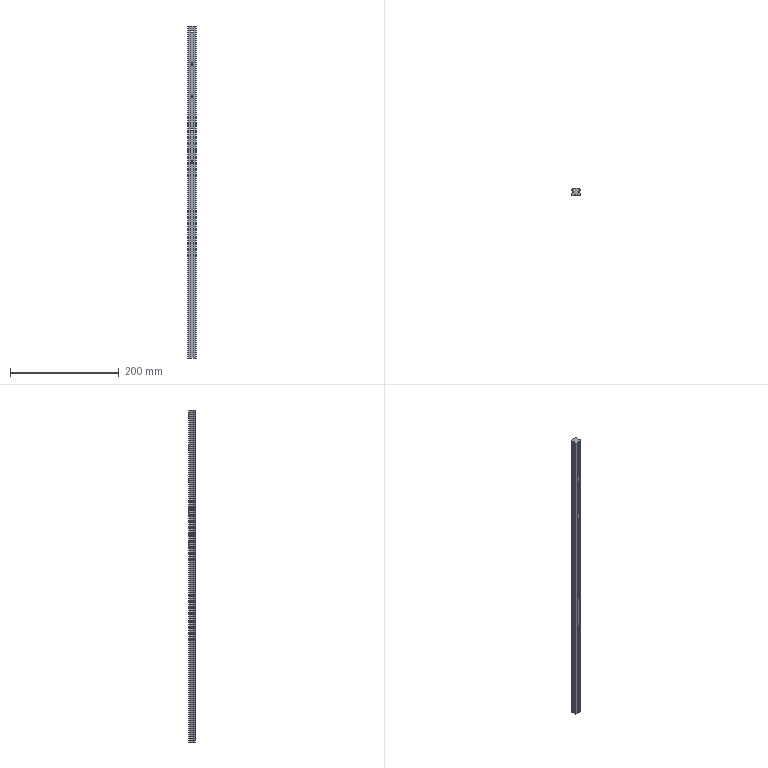Part | NX | 1 solid | 56 faces | box 15 x 12.5 x 610 mm | volume 97842 mm3 | plane 30 | cylinder 26 | commonest cylinder face diameters 0.6 x10 4.5 x5 8 x5 3 x4 1 x2